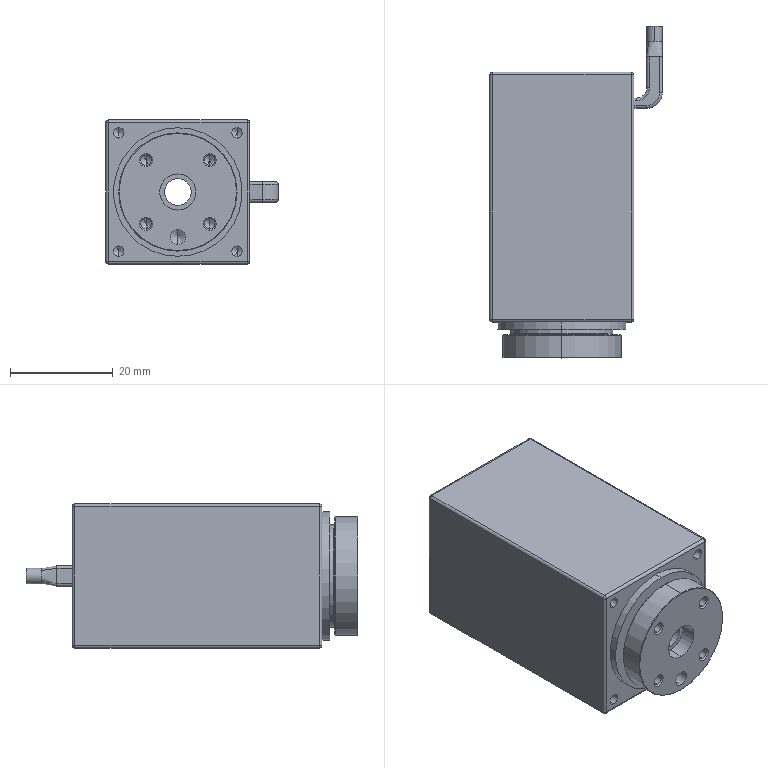Part | STEP file | 8 solids | 182 faces | box 33.5 x 64.5 x 28 mm | volume 32538 mm3 | cylinder 96 | plane 40 | cone 32 | sphere 8 | torus 4 | spline 2 | commonest cylinder face diameters 1 x20 2.05 x16 15 x10 7 x6 7.02 x6 16 x6